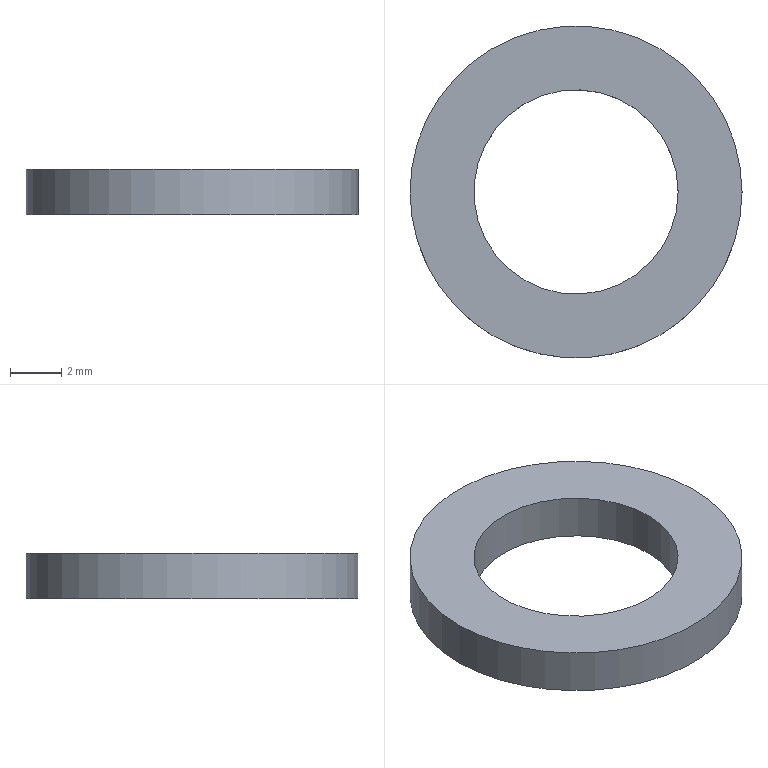Part | NX | features solid 2 | 1 solid | 4 faces | box 13 x 13 x 1.8 mm | volume 148.44 mm3 | plane 2 | cylinder 2 | commonest cylinder face diameters 8 x1 13 x1
STEP:
#1=CARTESIAN_POINT('',(46.5,30.,-71.8));
#2=VERTEX_POINT('',#1);
#3=CARTESIAN_POINT('',(40.,30.,-71.8));
#4=DIRECTION('',(0.,0.,1.));
#5=DIRECTION('',(1.,0.,0.));
#6=AXIS2_PLACEMENT_3D('',#3,#4,#5);
#7=CIRCLE('',#6,6.5);
#8=EDGE_CURVE('',#2,#2,#7,.T.);
#9=ORIENTED_EDGE('',*,*,#8,.F.);
#10=EDGE_LOOP('',(#9));
#11=FACE_BOUND('',#10,.T.);
#12=CARTESIAN_POINT('',(44.,30.,-71.8));
#13=VERTEX_POINT('',#12);
#14=CARTESIAN_POINT('',(40.,30.,-71.8));
#15=DIRECTION('',(0.,0.,1.));
#16=DIRECTION('',(1.,0.,0.));
#17=AXIS2_PLACEMENT_3D('',#14,#15,#16);
#18=CIRCLE('',#17,4.);
#19=EDGE_CURVE('',#13,#13,#18,.T.);
#20=ORIENTED_EDGE('',*,*,#19,.T.);
#21=EDGE_LOOP('',(#20));
#22=FACE_BOUND('',#21,.T.);
#23=CARTESIAN_POINT('',(40.,30.,-71.8));
#24=DIRECTION('',(0.,0.,-1.));
#25=DIRECTION('',(-1.,0.,0.));
#26=AXIS2_PLACEMENT_3D('',#23,#24,#25);
#27=PLANE('',#26);
#28=ADVANCED_FACE('',(#11,#22),#27,.T.);
#29=CARTESIAN_POINT('',(46.5,30.,-70.));
#30=VERTEX_POINT('',#29);
#31=CARTESIAN_POINT('',(40.,30.,-70.));
#32=DIRECTION('',(0.,0.,-1.));
#33=DIRECTION('',(1.,0.,0.));
#34=AXIS2_PLACEMENT_3D('',#31,#32,#33);
#35=CIRCLE('',#34,6.5);
#36=EDGE_CURVE('',#30,#30,#35,.T.);
#37=ORIENTED_EDGE('',*,*,#36,.F.);
#38=EDGE_LOOP('',(#37));
#39=FACE_BOUND('',#38,.T.);
#40=CARTESIAN_POINT('',(44.,30.,-70.));
#41=VERTEX_POINT('',#40);
#42=CARTESIAN_POINT('',(40.,30.,-70.));
#43=DIRECTION('',(0.,0.,-1.));
#44=DIRECTION('',(1.,0.,0.));
#45=AXIS2_PLACEMENT_3D('',#42,#43,#44);
#46=CIRCLE('',#45,4.);
#47=EDGE_CURVE('',#41,#41,#46,.T.);
#48=ORIENTED_EDGE('',*,*,#47,.T.);
#49=EDGE_LOOP('',(#48));
#50=FACE_BOUND('',#49,.T.);
#51=CARTESIAN_POINT('',(40.,30.,-70.));
#52=DIRECTION('',(0.,0.,1.));
#53=DIRECTION('',(1.,0.,0.));
#54=AXIS2_PLACEMENT_3D('',#51,#52,#53);
#55=PLANE('',#54);
#56=ADVANCED_FACE('',(#39,#50),#55,.T.);
#57=ORIENTED_EDGE('',*,*,#8,.T.);
#58=EDGE_LOOP('',(#57));
#59=FACE_BOUND('',#58,.T.);
#60=ORIENTED_EDGE('',*,*,#36,.T.);
#61=EDGE_LOOP('',(#60));
#62=FACE_BOUND('',#61,.T.);
#63=CARTESIAN_POINT('',(40.,30.,-70.));
#64=DIRECTION('',(0.,0.,-1.));
#65=DIRECTION('',(1.,0.,0.));
#66=AXIS2_PLACEMENT_3D('',#63,#64,#65);
#67=CYLINDRICAL_SURFACE('',#66,6.5);
#68=ADVANCED_FACE('',(#59,#62),#67,.T.);
#69=ORIENTED_EDGE('',*,*,#19,.F.);
#70=EDGE_LOOP('',(#69));
#71=FACE_BOUND('',#70,.T.);
#72=ORIENTED_EDGE('',*,*,#47,.F.);
#73=EDGE_LOOP('',(#72));
#74=FACE_BOUND('',#73,.T.);
#75=CARTESIAN_POINT('',(40.,30.,-70.));
#76=DIRECTION('',(0.,0.,-1.));
#77=DIRECTION('',(1.,0.,0.));
#78=AXIS2_PLACEMENT_3D('',#75,#76,#77);
#79=CYLINDRICAL_SURFACE('',#78,4.);
#80=ADVANCED_FACE('',(#71,#74),#79,.F.);
#81=CLOSED_SHELL('',(#28,#56,#68,#80));
#82=MANIFOLD_SOLID_BREP('',#81);
#83=(LENGTH_UNIT()NAMED_UNIT(*)SI_UNIT(.MILLI.,.METRE.));
#84=UNCERTAINTY_MEASURE_WITH_UNIT(LENGTH_MEASURE(0.00001),#83,'','');
#85=(NAMED_UNIT(*)PLANE_ANGLE_UNIT()SI_UNIT($,.RADIAN.));
#86=(NAMED_UNIT(*)SI_UNIT($,.STERADIAN.)SOLID_ANGLE_UNIT());
#87=(GEOMETRIC_REPRESENTATION_CONTEXT(3)GLOBAL_UNCERTAINTY_ASSIGNED_CONTEXT((#84))GLOBAL_UNIT_ASSIGNED_CONTEXT((#83,#85,#86))REPRESENTATION_CONTEXT('',''));
#88=ADVANCED_BREP_SHAPE_REPRESENTATION('',(#82),#87);